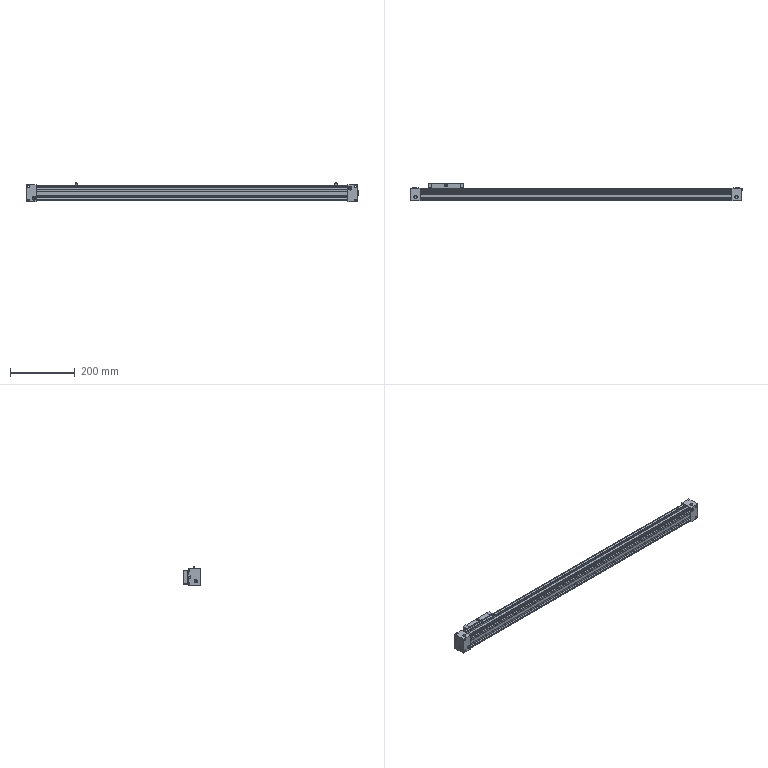Part | SolidWorks | 6 solids | 467 faces | box 1022 x 54 x 60.6 mm | volume 1632834 mm3 | plane 271 | cylinder 144 | cone 44 | spline 8 | commonest cylinder face diameters 2 x21 4.134 x12 4 x10 5.5 x8 5.6 x8 9 x8